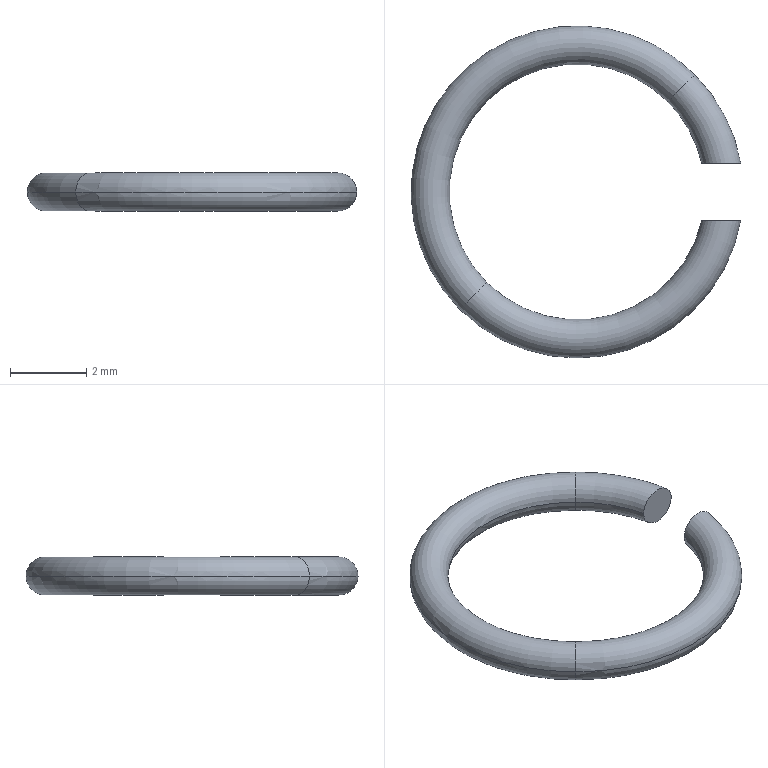Part | STEP file | ASND-0110-4216111400_AF0 | 1 solid | 8 faces | box 8.635 x 8.7 x 1 mm | volume 17.813 mm3 | torus 6 | plane 2
STEP:
#1=CARTESIAN_POINT('',(0.,0.,0.));
#2=DIRECTION('',(0.,0.,1.));
#3=DIRECTION('',(1.,0.,0.));
#4=AXIS2_PLACEMENT_3D('',#1,#2,#3);
#5=CARTESIAN_POINT('',(3.076,3.076,0.));
#6=VERTEX_POINT('',#5);
#7=CARTESIAN_POINT('',(2.369,2.369,0.));
#8=VERTEX_POINT('',#7);
#9=CARTESIAN_POINT('',(2.722,2.722,0.));
#10=DIRECTION('',(-0.7071,0.7071,0.));
#11=DIRECTION('',(-0.7071,-0.7071,0.));
#12=AXIS2_PLACEMENT_3D('',#9,#10,#11);
#13=CIRCLE('',#12,0.5);
#14=CARTESIAN_POINT('',(0.,0.,0.));
#15=DIRECTION('',(0.,0.,-1.));
#16=DIRECTION('',(0.7071,0.7071,0.));
#17=AXIS2_PLACEMENT_3D('',#14,#15,#16);
#18=TOROIDAL_SURFACE('',#17,3.85,0.5);
#19=CARTESIAN_POINT('',(0.,-3.142));
#20=DIRECTION('',(0.,1.));
#21=VECTOR('',#20,1.);
#22=LINE('',#19,#21);
#23=(GEOMETRIC_REPRESENTATION_CONTEXT(2)PARAMETRIC_REPRESENTATION_CONTEXT()REPRESENTATION_CONTEXT('',''));
#24=DEFINITIONAL_REPRESENTATION('',(#22),#23);
#25=PCURVE('',#18,#24);
#26=CARTESIAN_POINT('',(0.,0.,0.));
#27=DIRECTION('',(0.,0.,-1.));
#28=DIRECTION('',(0.7071,0.7071,0.));
#29=AXIS2_PLACEMENT_3D('',#26,#27,#28);
#30=TOROIDAL_SURFACE('',#29,3.85,0.5);
#31=CARTESIAN_POINT('',(6.283,-3.142));
#32=DIRECTION('',(0.,1.));
#33=VECTOR('',#32,1.);
#34=LINE('',#31,#33);
#35=(GEOMETRIC_REPRESENTATION_CONTEXT(2)PARAMETRIC_REPRESENTATION_CONTEXT()REPRESENTATION_CONTEXT('',''));
#36=DEFINITIONAL_REPRESENTATION('',(#34),#35);
#37=PCURVE('',#30,#36);
#38=SURFACE_CURVE('',#13,(#25,#37),.PCURVE_S1.);
#39=EDGE_CURVE('',#6,#8,#38,.T.);
#40=ORIENTED_EDGE('',*,*,#39,.F.);
#41=CARTESIAN_POINT('',(4.285,0.75,0.));
#42=VERTEX_POINT('',#41);
#43=CARTESIAN_POINT('',(0.,0.,0.));
#44=DIRECTION('',(0.,0.,-1.));
#45=DIRECTION('',(-1.,0.,0.));
#46=AXIS2_PLACEMENT_3D('',#43,#44,#45);
#47=CIRCLE('',#46,4.35);
#48=CARTESIAN_POINT('',(-2.356,0.));
#49=DIRECTION('',(1.,0.));
#50=VECTOR('',#49,1.);
#51=LINE('',#48,#50);
#52=(GEOMETRIC_REPRESENTATION_CONTEXT(2)PARAMETRIC_REPRESENTATION_CONTEXT()REPRESENTATION_CONTEXT('',''));
#53=DEFINITIONAL_REPRESENTATION('',(#51),#52);
#54=PCURVE('',#18,#53);
#55=CARTESIAN_POINT('',(0.,0.,0.));
#56=DIRECTION('',(0.,0.,-1.));
#57=DIRECTION('',(0.7071,0.7071,0.));
#58=AXIS2_PLACEMENT_3D('',#55,#56,#57);
#59=TOROIDAL_SURFACE('',#58,3.85,0.5);
#60=CARTESIAN_POINT('',(-2.356,6.283));
#61=DIRECTION('',(1.,0.));
#62=VECTOR('',#61,1.);
#63=LINE('',#60,#62);
#64=(GEOMETRIC_REPRESENTATION_CONTEXT(2)PARAMETRIC_REPRESENTATION_CONTEXT()REPRESENTATION_CONTEXT('',''));
#65=DEFINITIONAL_REPRESENTATION('',(#63),#64);
#66=PCURVE('',#59,#65);
#67=SURFACE_CURVE('',#47,(#54,#66),.PCURVE_S1.);
#68=EDGE_CURVE('',#6,#42,#67,.T.);
#69=ORIENTED_EDGE('',*,*,#68,.T.);
#70=CARTESIAN_POINT('',(3.776,0.75,-0.5));
#71=VERTEX_POINT('',#70);
#72=CARTESIAN_POINT('',(4.285,0.75,0.));
#73=CARTESIAN_POINT('',(4.285,0.75,-0.1146));
#74=CARTESIAN_POINT('',(4.242,0.7512,-0.2389));
#75=CARTESIAN_POINT('',(4.064,0.7514,-0.4328));
#76=CARTESIAN_POINT('',(3.926,0.75,-0.5));
#77=CARTESIAN_POINT('',(3.776,0.75,-0.5));
#78=B_SPLINE_CURVE_WITH_KNOTS('',3,(#72,#73,#74,#75,#76,#77),.UNSPECIFIED.,.F.,.F.,(4,2,4),(0.5,0.75,1.),.UNSPECIFIED.);
#79=CARTESIAN_POINT('',(0.6121,0.));
#80=CARTESIAN_POINT('',(0.6121,0.02083));
#81=CARTESIAN_POINT('',(0.6121,0.06282));
#82=CARTESIAN_POINT('',(0.6119,0.1267));
#83=CARTESIAN_POINT('',(0.6117,0.1915));
#84=CARTESIAN_POINT('',(0.6114,0.257));
#85=CARTESIAN_POINT('',(0.6109,0.3233));
#86=CARTESIAN_POINT('',(0.6104,0.3903));
#87=CARTESIAN_POINT('',(0.6098,0.4579));
#88=CARTESIAN_POINT('',(0.6091,0.5263));
#89=CARTESIAN_POINT('',(0.6083,0.5955));
#90=CARTESIAN_POINT('',(0.6074,0.6654));
#91=CARTESIAN_POINT('',(0.6064,0.7363));
#92=CARTESIAN_POINT('',(0.6054,0.8082));
#93=CARTESIAN_POINT('',(0.6042,0.881));
#94=CARTESIAN_POINT('',(0.6029,0.9547));
#95=CARTESIAN_POINT('',(0.6015,1.029));
#96=CARTESIAN_POINT('',(0.6001,1.104));
#97=CARTESIAN_POINT('',(0.5985,1.18));
#98=CARTESIAN_POINT('',(0.5969,1.257));
#99=CARTESIAN_POINT('',(0.5951,1.334));
#100=CARTESIAN_POINT('',(0.5933,1.412));
#101=CARTESIAN_POINT('',(0.5914,1.491));
#102=CARTESIAN_POINT('',(0.59,1.544));
#103=CARTESIAN_POINT('',(0.5893,1.571));
#104=B_SPLINE_CURVE_WITH_KNOTS('',3,(#79,#80,#81,#82,#83,#84,#85,#86,#87,#88,#89,#90,#91,#92,#93,#94,#95,#96,#97,#98,#99,#100,#101,#102,#103),.UNSPECIFIED.,.F.,.F.,(4,1,1,1,1,1,1,1,1,1,1,1,1,1,1,1,1,1,1,1,1,1,4),(0.5,0.5227,0.5455,0.5682,0.5909,0.6136,0.6364,0.6591,0.6818,0.7045,0.7273,0.75,0.7727,0.7955,0.8182,0.8409,0.8636,0.8864,0.9091,0.9318,0.9545,0.9773,1.),.QUASI_UNIFORM_KNOTS.);
#105=(GEOMETRIC_REPRESENTATION_CONTEXT(2)PARAMETRIC_REPRESENTATION_CONTEXT()REPRESENTATION_CONTEXT('',''));
#106=DEFINITIONAL_REPRESENTATION('',(#104),#105);
#107=PCURVE('',#18,#106);
#108=CARTESIAN_POINT('',(5.049,0.75,-1.526));
#109=DIRECTION('',(0.,1.,0.));
#110=DIRECTION('',(0.7071,0.,0.7071));
#111=AXIS2_PLACEMENT_3D('',#108,#109,#110);
#112=PLANE('',#111);
#113=CARTESIAN_POINT('',(0.5386,-1.619));
#114=CARTESIAN_POINT('',(0.4576,-1.538));
#115=CARTESIAN_POINT('',(0.3397,-1.48));
#116=CARTESIAN_POINT('',(0.07614,-1.469));
#117=CARTESIAN_POINT('',(-0.06847,-1.519));
#118=CARTESIAN_POINT('',(-0.1746,-1.625));
#119=B_SPLINE_CURVE_WITH_KNOTS('',3,(#113,#114,#115,#116,#117,#118),.UNSPECIFIED.,.F.,.F.,(4,2,4),(0.5,0.75,1.),.UNSPECIFIED.);
#120=(GEOMETRIC_REPRESENTATION_CONTEXT(2)PARAMETRIC_REPRESENTATION_CONTEXT()REPRESENTATION_CONTEXT('',''));
#121=DEFINITIONAL_REPRESENTATION('',(#119),#120);
#122=PCURVE('',#112,#121);
#123=SURFACE_CURVE('',#78,(#107,#122),.PCURVE_S1.);
#124=EDGE_CURVE('',#42,#71,#123,.T.);
#125=ORIENTED_EDGE('',*,*,#124,.T.);
#126=CARTESIAN_POINT('',(3.265,0.75,0.));
#127=VERTEX_POINT('',#126);
#128=CARTESIAN_POINT('',(3.776,0.75,-0.5));
#129=CARTESIAN_POINT('',(3.752,0.7499,-0.499));
#130=CARTESIAN_POINT('',(3.706,0.7499,-0.4972));
#131=CARTESIAN_POINT('',(3.642,0.7494,-0.4836));
#132=CARTESIAN_POINT('',(3.587,0.749,-0.4654));
#133=CARTESIAN_POINT('',(3.541,0.7488,-0.4445));
#134=CARTESIAN_POINT('',(3.503,0.7488,-0.4231));
#135=CARTESIAN_POINT('',(3.474,0.749,-0.4029));
#136=CARTESIAN_POINT('',(3.451,0.7493,-0.3853));
#137=CARTESIAN_POINT('',(3.434,0.7496,-0.3714));
#138=CARTESIAN_POINT('',(3.424,0.7499,-0.3617));
#139=CARTESIAN_POINT('',(3.384,0.7505,-0.3243));
#140=CARTESIAN_POINT('',(3.327,0.7495,-0.2494));
#141=CARTESIAN_POINT('',(3.274,0.7498,-0.1259));
#142=CARTESIAN_POINT('',(3.268,0.7499,-0.04095));
#143=CARTESIAN_POINT('',(3.265,0.75,0.));
#144=B_SPLINE_CURVE_WITH_KNOTS('',3,(#128,#129,#130,#131,#132,#133,#134,#135,#136,#137,#138,#139,#140,#141,#142,#143),.UNSPECIFIED.,.F.,.F.,(4,1,1,1,1,1,1,1,1,1,1,1,1,4),(0.,0.04566,0.08672,0.1232,0.1551,0.1824,0.2052,0.2234,0.237,0.246,0.2505,0.3396,0.4227,0.5),.UNSPECIFIED.);
#145=CARTESIAN_POINT('',(0.5893,1.571));
#146=CARTESIAN_POINT('',(0.5891,1.579));
#147=CARTESIAN_POINT('',(0.5887,1.594));
#148=CARTESIAN_POINT('',(0.5881,1.618));
#149=CARTESIAN_POINT('',(0.5875,1.642));
#150=CARTESIAN_POINT('',(0.5869,1.665));
#151=CARTESIAN_POINT('',(0.5863,1.689));
#152=CARTESIAN_POINT('',(0.5857,1.712));
#153=CARTESIAN_POINT('',(0.5851,1.736));
#154=CARTESIAN_POINT('',(0.5845,1.759));
#155=CARTESIAN_POINT('',(0.5839,1.783));
#156=CARTESIAN_POINT('',(0.5833,1.807));
#157=CARTESIAN_POINT('',(0.5826,1.83));
#158=CARTESIAN_POINT('',(0.582,1.854));
#159=CARTESIAN_POINT('',(0.5814,1.878));
#160=CARTESIAN_POINT('',(0.5808,1.901));
#161=CARTESIAN_POINT('',(0.5802,1.925));
#162=CARTESIAN_POINT('',(0.5796,1.948));
#163=CARTESIAN_POINT('',(0.579,1.972));
#164=CARTESIAN_POINT('',(0.5784,1.996));
#165=CARTESIAN_POINT('',(0.5778,2.019));
#166=CARTESIAN_POINT('',(0.5772,2.043));
#167=CARTESIAN_POINT('',(0.5766,2.066));
#168=CARTESIAN_POINT('',(0.576,2.09));
#169=CARTESIAN_POINT('',(0.5754,2.114));
#170=CARTESIAN_POINT('',(0.5748,2.137));
#171=CARTESIAN_POINT('',(0.5741,2.161));
#172=CARTESIAN_POINT('',(0.5735,2.185));
#173=CARTESIAN_POINT('',(0.5729,2.208));
#174=CARTESIAN_POINT('',(0.5723,2.232));
#175=CARTESIAN_POINT('',(0.5717,2.256));
#176=CARTESIAN_POINT('',(0.5711,2.279));
#177=CARTESIAN_POINT('',(0.5705,2.303));
#178=CARTESIAN_POINT('',(0.5699,2.326));
#179=CARTESIAN_POINT('',(0.5693,2.35));
#180=CARTESIAN_POINT('',(0.5688,2.374));
#181=CARTESIAN_POINT('',(0.5683,2.398));
#182=CARTESIAN_POINT('',(0.5677,2.421));
#183=CARTESIAN_POINT('',(0.5672,2.445));
#184=CARTESIAN_POINT('',(0.5668,2.469));
#185=CARTESIAN_POINT('',(0.5663,2.493));
#186=CARTESIAN_POINT('',(0.5659,2.517));
#187=CARTESIAN_POINT('',(0.5654,2.541));
#188=CARTESIAN_POINT('',(0.565,2.565));
#189=CARTESIAN_POINT('',(0.5646,2.589));
#190=CARTESIAN_POINT('',(0.5642,2.613));
#191=CARTESIAN_POINT('',(0.5639,2.637));
#192=CARTESIAN_POINT('',(0.5635,2.661));
#193=CARTESIAN_POINT('',(0.5631,2.685));
#194=CARTESIAN_POINT('',(0.5628,2.709));
#195=CARTESIAN_POINT('',(0.5625,2.733));
#196=CARTESIAN_POINT('',(0.5621,2.757));
#197=CARTESIAN_POINT('',(0.5618,2.781));
#198=CARTESIAN_POINT('',(0.5616,2.805));
#199=CARTESIAN_POINT('',(0.5613,2.829));
#200=CARTESIAN_POINT('',(0.5611,2.853));
#201=CARTESIAN_POINT('',(0.5608,2.877));
#202=CARTESIAN_POINT('',(0.5606,2.901));
#203=CARTESIAN_POINT('',(0.5605,2.925));
#204=CARTESIAN_POINT('',(0.5603,2.949));
#205=CARTESIAN_POINT('',(0.5602,2.973));
#206=CARTESIAN_POINT('',(0.5601,2.997));
#207=CARTESIAN_POINT('',(0.56,3.021));
#208=CARTESIAN_POINT('',(0.5599,3.045));
#209=CARTESIAN_POINT('',(0.5598,3.069));
#210=CARTESIAN_POINT('',(0.5597,3.093));
#211=CARTESIAN_POINT('',(0.5597,3.117));
#212=CARTESIAN_POINT('',(0.5596,3.134));
#213=CARTESIAN_POINT('',(0.5596,3.142));
#214=B_SPLINE_CURVE_WITH_KNOTS('',3,(#145,#146,#147,#148,#149,#150,#151,#152,#153,#154,#155,#156,#157,#158,#159,#160,#161,#162,#163,#164,#165,#166,#167,#168,#169,#170,#171,#172,#173,#174,#175,#176,#177,#178,#179,#180,#181,#182,#183,#184,#185,#186,#187,#188,#189,#190,#191,#192,#193,#194,#195,#196,#197,#198,#199,#200,#201,#202,#203,#204,#205,#206,#207,#208,#209,#210,#211,#212,#213),.UNSPECIFIED.,.F.,.F.,(4,1,1,1,1,1,1,1,1,1,1,1,1,1,1,1,1,1,1,1,1,1,1,1,1,1,1,1,1,1,1,1,1,1,1,1,1,1,1,1,1,1,1,1,1,1,1,1,1,1,1,1,1,1,1,1,1,1,1,1,1,1,1,1,1,1,4),(0.,0.007576,0.01515,0.02273,0.0303,0.03788,0.04545,0.05303,0.06061,0.06818,0.07576,0.08333,0.09091,0.09848,0.1061,0.1136,0.1212,0.1288,0.1364,0.1439,0.1515,0.1591,0.1667,0.1742,0.1818,0.1894,0.197,0.2045,0.2121,0.2197,0.2273,0.2348,0.2424,0.25,0.2576,0.2652,0.2727,0.2803,0.2879,0.2955,0.303,0.3106,0.3182,0.3258,0.3333,0.3409,0.3485,0.3561,0.3636,0.3712,0.3788,0.3864,0.3939,0.4015,0.4091,0.4167,0.4242,0.4318,0.4394,0.447,0.4545,0.4621,0.4697,0.4773,0.4848,0.4924,0.5),.QUASI_UNIFORM_KNOTS.);
#215=(GEOMETRIC_REPRESENTATION_CONTEXT(2)PARAMETRIC_REPRESENTATION_CONTEXT()REPRESENTATION_CONTEXT('',''));
#216=DEFINITIONAL_REPRESENTATION('',(#214),#215);
#217=PCURVE('',#18,#216);
#218=CARTESIAN_POINT('',(-0.1746,-1.625));
#219=CARTESIAN_POINT('',(-0.191,-1.643));
#220=CARTESIAN_POINT('',(-0.2221,-1.676));
#221=CARTESIAN_POINT('',(-0.2577,-1.731));
#222=CARTESIAN_POINT('',(-0.2838,-1.783));
#223=CARTESIAN_POINT('',(-0.3016,-1.83));
#224=CARTESIAN_POINT('',(-0.3131,-1.872));
#225=CARTESIAN_POINT('',(-0.32,-1.908));
#226=CARTESIAN_POINT('',(-0.3238,-1.936));
#227=CARTESIAN_POINT('',(-0.3255,-1.958));
#228=CARTESIAN_POINT('',(-0.3262,-1.972));
#229=CARTESIAN_POINT('',(-0.3275,-2.026));
#230=CARTESIAN_POINT('',(-0.3154,-2.12));
#231=CARTESIAN_POINT('',(-0.265,-2.244));
#232=CARTESIAN_POINT('',(-0.2094,-2.309));
#233=CARTESIAN_POINT('',(-0.1826,-2.34));
#234=B_SPLINE_CURVE_WITH_KNOTS('',3,(#218,#219,#220,#221,#222,#223,#224,#225,#226,#227,#228,#229,#230,#231,#232,#233),.UNSPECIFIED.,.F.,.F.,(4,1,1,1,1,1,1,1,1,1,1,1,1,4),(0.,0.04566,0.08672,0.1232,0.1551,0.1824,0.2052,0.2234,0.237,0.246,0.2505,0.3396,0.4227,0.5),.UNSPECIFIED.);
#235=(GEOMETRIC_REPRESENTATION_CONTEXT(2)PARAMETRIC_REPRESENTATION_CONTEXT()REPRESENTATION_CONTEXT('',''));
#236=DEFINITIONAL_REPRESENTATION('',(#234),#235);
#237=PCURVE('',#112,#236);
#238=SURFACE_CURVE('',#144,(#217,#237),.PCURVE_S1.);
#239=EDGE_CURVE('',#71,#127,#238,.T.);
#240=ORIENTED_EDGE('',*,*,#239,.T.);
#241=CARTESIAN_POINT('',(0.,0.,0.));
#242=DIRECTION('',(0.,0.,-1.));
#243=DIRECTION('',(-1.,0.,0.));
#244=AXIS2_PLACEMENT_3D('',#241,#242,#243);
#245=CIRCLE('',#244,3.35);
#246=CARTESIAN_POINT('',(-2.356,3.142));
#247=DIRECTION('',(1.,0.));
#248=VECTOR('',#247,1.);
#249=LINE('',#246,#248);
#250=(GEOMETRIC_REPRESENTATION_CONTEXT(2)PARAMETRIC_REPRESENTATION_CONTEXT()REPRESENTATION_CONTEXT('',''));
#251=DEFINITIONAL_REPRESENTATION('',(#249),#250);
#252=PCURVE('',#18,#251);
#253=CARTESIAN_POINT('',(-2.356,3.142));
#254=DIRECTION('',(1.,0.));
#255=VECTOR('',#254,1.);
#256=LINE('',#253,#255);
#257=(GEOMETRIC_REPRESENTATION_CONTEXT(2)PARAMETRIC_REPRESENTATION_CONTEXT()REPRESENTATION_CONTEXT('',''));
#258=DEFINITIONAL_REPRESENTATION('',(#256),#257);
#259=PCURVE('',#59,#258);
#260=SURFACE_CURVE('',#245,(#252,#259),.PCURVE_S1.);
#261=EDGE_CURVE('',#8,#127,#260,.T.);
#262=ORIENTED_EDGE('',*,*,#261,.F.);
#263=EDGE_LOOP('',(#40,#69,#125,#240,#262));
#264=FACE_BOUND('',#263,.T.);
#265=ADVANCED_FACE('',(#264),#18,.T.);
#266=CARTESIAN_POINT('',(-3.076,-3.076,0.));
#267=VERTEX_POINT('',#266);
#268=CARTESIAN_POINT('',(-2.369,-2.369,0.));
#269=VERTEX_POINT('',#268);
#270=CARTESIAN_POINT('',(-2.722,-2.722,0.));
#271=DIRECTION('',(0.7071,-0.7071,0.));
#272=DIRECTION('',(0.7071,0.7071,0.));
#273=AXIS2_PLACEMENT_3D('',#270,#271,#272);
#274=CIRCLE('',#273,0.5);
#275=CARTESIAN_POINT('',(3.142,-3.142));
#276=DIRECTION('',(0.,1.));
#277=VECTOR('',#276,1.);
#278=LINE('',#275,#277);
#279=(GEOMETRIC_REPRESENTATION_CONTEXT(2)PARAMETRIC_REPRESENTATION_CONTEXT()REPRESENTATION_CONTEXT('',''));
#280=DEFINITIONAL_REPRESENTATION('',(#278),#279);
#281=PCURVE('',#30,#280);
#282=CARTESIAN_POINT('',(0.,0.,0.));
#283=DIRECTION('',(0.,0.,-1.));
#284=DIRECTION('',(0.7071,0.7071,0.));
#285=AXIS2_PLACEMENT_3D('',#282,#283,#284);
#286=TOROIDAL_SURFACE('',#285,3.85,0.5);
#287=CARTESIAN_POINT('',(3.142,-3.142));
#288=DIRECTION('',(0.,1.));
#289=VECTOR('',#288,1.);
#290=LINE('',#287,#289);
#291=(GEOMETRIC_REPRESENTATION_CONTEXT(2)PARAMETRIC_REPRESENTATION_CONTEXT()REPRESENTATION_CONTEXT('',''));
#292=DEFINITIONAL_REPRESENTATION('',(#290),#291);
#293=PCURVE('',#286,#292);
#294=SURFACE_CURVE('',#274,(#281,#293),.PCURVE_S1.);
#295=EDGE_CURVE('',#267,#269,#294,.T.);
#296=ORIENTED_EDGE('',*,*,#295,.F.);
#297=CARTESIAN_POINT('',(0.,0.,0.));
#298=DIRECTION('',(0.,0.,-1.));
#299=DIRECTION('',(-1.,0.,0.));
#300=AXIS2_PLACEMENT_3D('',#297,#298,#299);
#301=CIRCLE('',#300,4.35);
#302=CARTESIAN_POINT('',(-2.356,0.));
#303=DIRECTION('',(1.,0.));
#304=VECTOR('',#303,1.);
#305=LINE('',#302,#304);
#306=(GEOMETRIC_REPRESENTATION_CONTEXT(2)PARAMETRIC_REPRESENTATION_CONTEXT()REPRESENTATION_CONTEXT('',''));
#307=DEFINITIONAL_REPRESENTATION('',(#305),#306);
#308=PCURVE('',#30,#307);
#309=CARTESIAN_POINT('',(0.,0.,0.));
#310=DIRECTION('',(0.,0.,-1.));
#311=DIRECTION('',(0.7071,0.7071,0.));
#312=AXIS2_PLACEMENT_3D('',#309,#310,#311);
#313=TOROIDAL_SURFACE('',#312,3.85,0.5);
#314=CARTESIAN_POINT('',(-2.356,6.283));
#315=DIRECTION('',(1.,0.));
#316=VECTOR('',#315,1.);
#317=LINE('',#314,#316);
#318=(GEOMETRIC_REPRESENTATION_CONTEXT(2)PARAMETRIC_REPRESENTATION_CONTEXT()REPRESENTATION_CONTEXT('',''));
#319=DEFINITIONAL_REPRESENTATION('',(#317),#318);
#320=PCURVE('',#313,#319);
#321=SURFACE_CURVE('',#301,(#308,#320),.PCURVE_S1.);
#322=EDGE_CURVE('',#267,#6,#321,.T.);
#323=ORIENTED_EDGE('',*,*,#322,.T.);
#324=ORIENTED_EDGE('',*,*,#39,.T.);
#325=CARTESIAN_POINT('',(0.,0.,0.));
#326=DIRECTION('',(0.,0.,-1.));
#327=DIRECTION('',(-1.,0.,0.));
#328=AXIS2_PLACEMENT_3D('',#325,#326,#327);
#329=CIRCLE('',#328,3.35);
#330=CARTESIAN_POINT('',(-2.356,3.142));
#331=DIRECTION('',(1.,0.));
#332=VECTOR('',#331,1.);
#333=LINE('',#330,#332);
#334=(GEOMETRIC_REPRESENTATION_CONTEXT(2)PARAMETRIC_REPRESENTATION_CONTEXT()REPRESENTATION_CONTEXT('',''));
#335=DEFINITIONAL_REPRESENTATION('',(#333),#334);
#336=PCURVE('',#30,#335);
#337=CARTESIAN_POINT('',(-2.356,3.142));
#338=DIRECTION('',(1.,0.));
#339=VECTOR('',#338,1.);
#340=LINE('',#337,#339);
#341=(GEOMETRIC_REPRESENTATION_CONTEXT(2)PARAMETRIC_REPRESENTATION_CONTEXT()REPRESENTATION_CONTEXT('',''));
#342=DEFINITIONAL_REPRESENTATION('',(#340),#341);
#343=PCURVE('',#313,#342);
#344=SURFACE_CURVE('',#329,(#336,#343),.PCURVE_S1.);
#345=EDGE_CURVE('',#269,#8,#344,.T.);
#346=ORIENTED_EDGE('',*,*,#345,.F.);
#347=EDGE_LOOP('',(#296,#323,#324,#346));
#348=FACE_BOUND('',#347,.T.);
#349=ADVANCED_FACE('',(#348),#30,.T.);
#350=CARTESIAN_POINT('',(3.776,-0.75,-0.5));
#351=VERTEX_POINT('',#350);
#352=CARTESIAN_POINT('',(4.285,-0.75,0.));
#353=VERTEX_POINT('',#352);
#354=CARTESIAN_POINT('',(3.776,-0.75,-0.5));
#355=CARTESIAN_POINT('',(3.926,-0.75,-0.5));
#356=CARTESIAN_POINT('',(4.064,-0.7514,-0.4328));
#357=CARTESIAN_POINT('',(4.242,-0.7512,-0.2389));
#358=CARTESIAN_POINT('',(4.285,-0.75,-0.1146));
#359=CARTESIAN_POINT('',(4.285,-0.75,0.));
#360=B_SPLINE_CURVE_WITH_KNOTS('',3,(#354,#355,#356,#357,#358,#359),.UNSPECIFIED.,.F.,.F.,(4,2,4),(0.,0.25,0.5),.UNSPECIFIED.);
#361=CARTESIAN_POINT('',(0.9815,1.571));
#362=CARTESIAN_POINT('',(0.9808,1.544));
#363=CARTESIAN_POINT('',(0.9794,1.491));
#364=CARTESIAN_POINT('',(0.9775,1.412));
#365=CARTESIAN_POINT('',(0.9757,1.334));
#366=CARTESIAN_POINT('',(0.9739,1.257));
#367=CARTESIAN_POINT('',(0.9723,1.18));
#368=CARTESIAN_POINT('',(0.9707,1.105));
#369=CARTESIAN_POINT('',(0.9693,1.029));
#370=CARTESIAN_POINT('',(0.9679,0.9548));
#371=CARTESIAN_POINT('',(0.9666,0.8811));
#372=CARTESIAN_POINT('',(0.9654,0.8083));
#373=CARTESIAN_POINT('',(0.9644,0.7364));
#374=CARTESIAN_POINT('',(0.9634,0.6655));
#375=CARTESIAN_POINT('',(0.9625,0.5956));
#376=CARTESIAN_POINT('',(0.9617,0.5264));
#377=CARTESIAN_POINT('',(0.961,0.458));
#378=CARTESIAN_POINT('',(0.9604,0.3903));
#379=CARTESIAN_POINT('',(0.9599,0.3233));
#380=CARTESIAN_POINT('',(0.9594,0.257));
#381=CARTESIAN_POINT('',(0.9591,0.1915));
#382=CARTESIAN_POINT('',(0.9589,0.1267));
#383=CARTESIAN_POINT('',(0.9587,0.06282));
#384=CARTESIAN_POINT('',(0.9587,0.02083));
#385=CARTESIAN_POINT('',(0.9587,0.));
#386=B_SPLINE_CURVE_WITH_KNOTS('',3,(#361,#362,#363,#364,#365,#366,#367,#368,#369,#370,#371,#372,#373,#374,#375,#376,#377,#378,#379,#380,#381,#382,#383,#384,#385),.UNSPECIFIED.,.F.,.F.,(4,1,1,1,1,1,1,1,1,1,1,1,1,1,1,1,1,1,1,1,1,1,4),(0.,0.02273,0.04545,0.06818,0.09091,0.1136,0.1364,0.1591,0.1818,0.2045,0.2273,0.25,0.2727,0.2955,0.3182,0.3409,0.3636,0.3864,0.4091,0.4318,0.4545,0.4773,0.5),.QUASI_UNIFORM_KNOTS.);
#387=(GEOMETRIC_REPRESENTATION_CONTEXT(2)PARAMETRIC_REPRESENTATION_CONTEXT()REPRESENTATION_CONTEXT('',''));
#388=DEFINITIONAL_REPRESENTATION('',(#386),#387);
#389=PCURVE('',#286,#388);
#390=CARTESIAN_POINT('',(2.042,-0.75,-1.526));
#391=DIRECTION('',(0.,-1.,0.));
#392=DIRECTION('',(0.7071,0.,0.7071));
#393=AXIS2_PLACEMENT_3D('',#390,#391,#392);
#394=PLANE('',#393);
#395=CARTESIAN_POINT('',(1.951,-0.501));
#396=CARTESIAN_POINT('',(2.057,-0.6071));
#397=CARTESIAN_POINT('',(2.202,-0.6567));
#398=CARTESIAN_POINT('',(2.465,-0.646));
#399=CARTESIAN_POINT('',(2.583,-0.5881));
#400=CARTESIAN_POINT('',(2.664,-0.5071));
#401=B_SPLINE_CURVE_WITH_KNOTS('',3,(#395,#396,#397,#398,#399,#400),.UNSPECIFIED.,.F.,.F.,(4,2,4),(0.,0.25,0.5),.UNSPECIFIED.);
#402=(GEOMETRIC_REPRESENTATION_CONTEXT(2)PARAMETRIC_REPRESENTATION_CONTEXT()REPRESENTATION_CONTEXT('',''));
#403=DEFINITIONAL_REPRESENTATION('',(#401),#402);
#404=PCURVE('',#394,#403);
#405=SURFACE_CURVE('',#360,(#389,#404),.PCURVE_S1.);
#406=EDGE_CURVE('',#351,#353,#405,.T.);
#407=ORIENTED_EDGE('',*,*,#406,.T.);
#408=CARTESIAN_POINT('',(0.,0.,0.));
#409=DIRECTION('',(0.,0.,-1.));
#410=DIRECTION('',(-1.,0.,0.));
#411=AXIS2_PLACEMENT_3D('',#408,#409,#410);
#412=CIRCLE('',#411,4.35);
#413=CARTESIAN_POINT('',(-2.356,0.));
#414=DIRECTION('',(1.,0.));
#415=VECTOR('',#414,1.);
#416=LINE('',#413,#415);
#417=(GEOMETRIC_REPRESENTATION_CONTEXT(2)PARAMETRIC_REPRESENTATION_CONTEXT()REPRESENTATION_CONTEXT('',''));
#418=DEFINITIONAL_REPRESENTATION('',(#416),#417);
#419=PCURVE('',#286,#418);
#420=CARTESIAN_POINT('',(0.,0.,0.));
#421=DIRECTION('',(0.,0.,-1.));
#422=DIRECTION('',(0.7071,0.7071,0.));
#423=AXIS2_PLACEMENT_3D('',#420,#421,#422);
#424=TOROIDAL_SURFACE('',#423,3.85,0.5);
#425=CARTESIAN_POINT('',(-2.356,6.283));
#426=DIRECTION('',(1.,0.));
#427=VECTOR('',#426,1.);
#428=LINE('',#425,#427);
#429=(GEOMETRIC_REPRESENTATION_CONTEXT(2)PARAMETRIC_REPRESENTATION_CONTEXT()REPRESENTATION_CONTEXT('',''));
#430=DEFINITIONAL_REPRESENTATION('',(#428),#429);
#431=PCURVE('',#424,#430);
#432=SURFACE_CURVE('',#412,(#419,#431),.PCURVE_S1.);
#433=EDGE_CURVE('',#353,#267,#432,.T.);
#434=ORIENTED_EDGE('',*,*,#433,.T.);
#435=ORIENTED_EDGE('',*,*,#295,.T.);
#436=CARTESIAN_POINT('',(3.265,-0.75,0.));
#437=VERTEX_POINT('',#436);
#438=CARTESIAN_POINT('',(0.,0.,0.));
#439=DIRECTION('',(0.,0.,-1.));
#440=DIRECTION('',(-1.,0.,0.));
#441=AXIS2_PLACEMENT_3D('',#438,#439,#440);
#442=CIRCLE('',#441,3.35);
#443=CARTESIAN_POINT('',(-2.356,3.142));
#444=DIRECTION('',(1.,0.));
#445=VECTOR('',#444,1.);
#446=LINE('',#443,#445);
#447=(GEOMETRIC_REPRESENTATION_CONTEXT(2)PARAMETRIC_REPRESENTATION_CONTEXT()REPRESENTATION_CONTEXT('',''));
#448=DEFINITIONAL_REPRESENTATION('',(#446),#447);
#449=PCURVE('',#286,#448);
#450=CARTESIAN_POINT('',(-2.356,3.142));
#451=DIRECTION('',(1.,0.));
#452=VECTOR('',#451,1.);
#453=LINE('',#450,#452);
#454=(GEOMETRIC_REPRESENTATION_CONTEXT(2)PARAMETRIC_REPRESENTATION_CONTEXT()REPRESENTATION_CONTEXT('',''));
#455=DEFINITIONAL_REPRESENTATION('',(#453),#454);
#456=PCURVE('',#424,#455);
#457=SURFACE_CURVE('',#442,(#449,#456),.PCURVE_S1.);
#458=EDGE_CURVE('',#437,#269,#457,.T.);
#459=ORIENTED_EDGE('',*,*,#458,.F.);
#460=CARTESIAN_POINT('',(3.265,-0.75,0.));
#461=CARTESIAN_POINT('',(3.266,-0.75,-0.02009));
#462=CARTESIAN_POINT('',(3.267,-0.7499,-0.06104));
#463=CARTESIAN_POINT('',(3.279,-0.7498,-0.1226));
#464=CARTESIAN_POINT('',(3.3,-0.7497,-0.1844));
#465=CARTESIAN_POINT('',(3.329,-0.7498,-0.245));
#466=CARTESIAN_POINT('',(3.368,-0.7499,-0.3032));
#467=CARTESIAN_POINT('',(3.423,-0.7503,-0.365));
#468=CARTESIAN_POINT('',(3.546,-0.7476,-0.4638));
#469=CARTESIAN_POINT('',(3.68,-0.749,-0.4848));
#470=CARTESIAN_POINT('',(3.776,-0.75,-0.5));
#471=B_SPLINE_CURVE_WITH_KNOTS('',3,(#460,#461,#462,#463,#464,#465,#466,#467,#468,#469,#470),.UNSPECIFIED.,.F.,.F.,(4,1,1,1,1,1,1,1,4),(0.5,0.5381,0.5777,0.6188,0.6613,0.7054,0.751,0.8192,1.),.UNSPECIFIED.);
#472=CARTESIAN_POINT('',(1.011,3.142));
#473=CARTESIAN_POINT('',(1.011,3.13));
#474=CARTESIAN_POINT('',(1.011,3.106));
#475=CARTESIAN_POINT('',(1.011,3.07));
#476=CARTESIAN_POINT('',(1.011,3.034));
#477=CARTESIAN_POINT('',(1.011,2.998));
#478=CARTESIAN_POINT('',(1.011,2.962));
#479=CARTESIAN_POINT('',(1.01,2.926));
#480=CARTESIAN_POINT('',(1.01,2.89));
#481=CARTESIAN_POINT('',(1.01,2.854));
#482=CARTESIAN_POINT('',(1.009,2.819));
#483=CARTESIAN_POINT('',(1.009,2.783));
#484=CARTESIAN_POINT('',(1.009,2.747));
#485=CARTESIAN_POINT('',(1.008,2.711));
#486=CARTESIAN_POINT('',(1.008,2.675));
#487=CARTESIAN_POINT('',(1.007,2.64));
#488=CARTESIAN_POINT('',(1.006,2.604));
#489=CARTESIAN_POINT('',(1.006,2.568));
#490=CARTESIAN_POINT('',(1.005,2.533));
#491=CARTESIAN_POINT('',(1.005,2.497));
#492=CARTESIAN_POINT('',(1.004,2.461));
#493=CARTESIAN_POINT('',(1.003,2.426));
#494=CARTESIAN_POINT('',(1.002,2.39));
#495=CARTESIAN_POINT('',(1.002,2.355));
#496=CARTESIAN_POINT('',(1.001,2.319));
#497=CARTESIAN_POINT('',(0.9999,2.284));
#498=CARTESIAN_POINT('',(0.999,2.248));
#499=CARTESIAN_POINT('',(0.998,2.213));
#500=CARTESIAN_POINT('',(0.9971,2.177));
#501=CARTESIAN_POINT('',(0.9962,2.142));
#502=CARTESIAN_POINT('',(0.9952,2.107));
#503=CARTESIAN_POINT('',(0.9943,2.073));
#504=CARTESIAN_POINT('',(0.9933,2.038));
#505=CARTESIAN_POINT('',(0.9924,2.003));
#506=CARTESIAN_POINT('',(0.9915,1.968));
#507=CARTESIAN_POINT('',(0.9905,1.932));
#508=CARTESIAN_POINT('',(0.9896,1.897));
#509=CARTESIAN_POINT('',(0.9887,1.861));
#510=CARTESIAN_POINT('',(0.9877,1.825));
#511=CARTESIAN_POINT('',(0.9868,1.789));
#512=CARTESIAN_POINT('',(0.9859,1.752));
#513=CARTESIAN_POINT('',(0.985,1.716));
#514=CARTESIAN_POINT('',(0.9841,1.68));
#515=CARTESIAN_POINT('',(0.9832,1.643));
#516=CARTESIAN_POINT('',(0.9823,1.607));
#517=CARTESIAN_POINT('',(0.9817,1.583));
#518=CARTESIAN_POINT('',(0.9815,1.571));
#519=B_SPLINE_CURVE_WITH_KNOTS('',3,(#472,#473,#474,#475,#476,#477,#478,#479,#480,#481,#482,#483,#484,#485,#486,#487,#488,#489,#490,#491,#492,#493,#494,#495,#496,#497,#498,#499,#500,#501,#502,#503,#504,#505,#506,#507,#508,#509,#510,#511,#512,#513,#514,#515,#516,#517,#518),.UNSPECIFIED.,.F.,.F.,(4,1,1,1,1,1,1,1,1,1,1,1,1,1,1,1,1,1,1,1,1,1,1,1,1,1,1,1,1,1,1,1,1,1,1,1,1,1,1,1,1,1,1,1,4),(0.5,0.5114,0.5227,0.5341,0.5455,0.5568,0.5682,0.5795,0.5909,0.6023,0.6136,0.625,0.6364,0.6477,0.6591,0.6705,0.6818,0.6932,0.7045,0.7159,0.7273,0.7386,0.75,0.7614,0.7727,0.7841,0.7955,0.8068,0.8182,0.8295,0.8409,0.8523,0.8636,0.875,0.8864,0.8977,0.9091,0.9205,0.9318,0.9432,0.9545,0.9659,0.9773,0.9886,1.),.QUASI_UNIFORM_KNOTS.);
#520=(GEOMETRIC_REPRESENTATION_CONTEXT(2)PARAMETRIC_REPRESENTATION_CONTEXT()REPRESENTATION_CONTEXT('',''));
#521=DEFINITIONAL_REPRESENTATION('',(#519),#520);
#522=PCURVE('',#286,#521);
#523=CARTESIAN_POINT('',(1.943,0.2141));
#524=CARTESIAN_POINT('',(1.93,0.1994));
#525=CARTESIAN_POINT('',(1.902,0.1694));
#526=CARTESIAN_POINT('',(1.867,0.1172));
#527=CARTESIAN_POINT('',(1.837,0.05924));
#528=CARTESIAN_POINT('',(1.815,-0.004466));
#529=CARTESIAN_POINT('',(1.802,-0.073));
#530=CARTESIAN_POINT('',(1.797,-0.1561));
#531=CARTESIAN_POINT('',(1.814,-0.313));
#532=CARTESIAN_POINT('',(1.894,-0.4219));
#533=CARTESIAN_POINT('',(1.951,-0.501));
#534=B_SPLINE_CURVE_WITH_KNOTS('',3,(#523,#524,#525,#526,#527,#528,#529,#530,#531,#532,#533),.UNSPECIFIED.,.F.,.F.,(4,1,1,1,1,1,1,1,4),(0.5,0.5381,0.5777,0.6188,0.6613,0.7054,0.751,0.8192,1.),.UNSPECIFIED.);
#535=(GEOMETRIC_REPRESENTATION_CONTEXT(2)PARAMETRIC_REPRESENTATION_CONTEXT()REPRESENTATION_CONTEXT('',''));
#536=DEFINITIONAL_REPRESENTATION('',(#534),#535);
#537=PCURVE('',#394,#536);
#538=SURFACE_CURVE('',#471,(#522,#537),.PCURVE_S1.);
#539=EDGE_CURVE('',#437,#351,#538,.T.);
#540=ORIENTED_EDGE('',*,*,#539,.T.);
#541=EDGE_LOOP('',(#407,#434,#435,#459,#540));
#542=FACE_BOUND('',#541,.T.);
#543=ADVANCED_FACE('',(#542),#286,.T.);
#544=ORIENTED_EDGE('',*,*,#433,.F.);
#545=CARTESIAN_POINT('',(3.776,-0.75,0.5));
#546=VERTEX_POINT('',#545);
#547=CARTESIAN_POINT('',(4.285,-0.75,0.));
#548=CARTESIAN_POINT('',(4.285,-0.75,0.1146));
#549=CARTESIAN_POINT('',(4.242,-0.7512,0.2389));
#550=CARTESIAN_POINT('',(4.064,-0.7514,0.4328));
#551=CARTESIAN_POINT('',(3.926,-0.75,0.5));
#552=CARTESIAN_POINT('',(3.776,-0.75,0.5));
#553=B_SPLINE_CURVE_WITH_KNOTS('',3,(#547,#548,#549,#550,#551,#552),.UNSPECIFIED.,.F.,.F.,(4,2,4),(0.5,0.75,1.),.UNSPECIFIED.);
#554=CARTESIAN_POINT('',(0.9587,6.283));
#555=CARTESIAN_POINT('',(0.9587,6.262));
#556=CARTESIAN_POINT('',(0.9587,6.22));
#557=CARTESIAN_POINT('',(0.9589,6.156));
#558=CARTESIAN_POINT('',(0.9591,6.092));
#559=CARTESIAN_POINT('',(0.9594,6.026));
#560=CARTESIAN_POINT('',(0.9598,5.96));
#561=CARTESIAN_POINT('',(0.9604,5.893));
#562=CARTESIAN_POINT('',(0.961,5.825));
#563=CARTESIAN_POINT('',(0.9617,5.757));
#564=CARTESIAN_POINT('',(0.9625,5.688));
#565=CARTESIAN_POINT('',(0.9634,5.618));
#566=CARTESIAN_POINT('',(0.9644,5.547));
#567=CARTESIAN_POINT('',(0.9654,5.475));
#568=CARTESIAN_POINT('',(0.9666,5.402));
#569=CARTESIAN_POINT('',(0.9679,5.329));
#570=CARTESIAN_POINT('',(0.9692,5.254));
#571=CARTESIAN_POINT('',(0.9707,5.179));
#572=CARTESIAN_POINT('',(0.9723,5.103));
#573=CARTESIAN_POINT('',(0.9739,5.026));
#574=CARTESIAN_POINT('',(0.9757,4.949));
#575=CARTESIAN_POINT('',(0.9775,4.871));
#576=CARTESIAN_POINT('',(0.9794,4.792));
#577=CARTESIAN_POINT('',(0.9808,4.739));
#578=CARTESIAN_POINT('',(0.9815,4.712));
#579=B_SPLINE_CURVE_WITH_KNOTS('',3,(#554,#555,#556,#557,#558,#559,#560,#561,#562,#563,#564,#565,#566,#567,#568,#569,#570,#571,#572,#573,#574,#575,#576,#577,#578),.UNSPECIFIED.,.F.,.F.,(4,1,1,1,1,1,1,1,1,1,1,1,1,1,1,1,1,1,1,1,1,1,4),(0.5,0.5227,0.5455,0.5682,0.5909,0.6136,0.6364,0.6591,0.6818,0.7045,0.7273,0.75,0.7727,0.7955,0.8182,0.8409,0.8636,0.8864,0.9091,0.9318,0.9545,0.9773,1.),.QUASI_UNIFORM_KNOTS.);
#580=(GEOMETRIC_REPRESENTATION_CONTEXT(2)PARAMETRIC_REPRESENTATION_CONTEXT()REPRESENTATION_CONTEXT('',''));
#581=DEFINITIONAL_REPRESENTATION('',(#579),#580);
#582=PCURVE('',#424,#581);
#583=CARTESIAN_POINT('',(2.664,-0.5071));
#584=CARTESIAN_POINT('',(2.745,-0.4261));
#585=CARTESIAN_POINT('',(2.803,-0.3082));
#586=CARTESIAN_POINT('',(2.814,-0.04462));
#587=CARTESIAN_POINT('',(2.765,0.09999));
#588=CARTESIAN_POINT('',(2.658,0.2061));
#589=B_SPLINE_CURVE_WITH_KNOTS('',3,(#583,#584,#585,#586,#587,#588),.UNSPECIFIED.,.F.,.F.,(4,2,4),(0.5,0.75,1.),.UNSPECIFIED.);
#590=(GEOMETRIC_REPRESENTATION_CONTEXT(2)PARAMETRIC_REPRESENTATION_CONTEXT()REPRESENTATION_CONTEXT('',''));
#591=DEFINITIONAL_REPRESENTATION('',(#589),#590);
#592=PCURVE('',#394,#591);
#593=SURFACE_CURVE('',#553,(#582,#592),.PCURVE_S1.);
#594=EDGE_CURVE('',#353,#546,#593,.T.);
#595=ORIENTED_EDGE('',*,*,#594,.T.);
#596=CARTESIAN_POINT('',(3.776,-0.75,0.5));
#597=CARTESIAN_POINT('',(3.752,-0.7499,0.499));
#598=CARTESIAN_POINT('',(3.706,-0.7499,0.4972));
#599=CARTESIAN_POINT('',(3.642,-0.7494,0.4836));
#600=CARTESIAN_POINT('',(3.587,-0.749,0.4654));
#601=CARTESIAN_POINT('',(3.541,-0.7488,0.4445));
#602=CARTESIAN_POINT('',(3.503,-0.7488,0.4231));
#603=CARTESIAN_POINT('',(3.474,-0.749,0.4029));
#604=CARTESIAN_POINT('',(3.451,-0.7493,0.3853));
#605=CARTESIAN_POINT('',(3.434,-0.7496,0.3714));
#606=CARTESIAN_POINT('',(3.424,-0.7499,0.3617));
#607=CARTESIAN_POINT('',(3.384,-0.7505,0.3243));
#608=CARTESIAN_POINT('',(3.327,-0.7495,0.2494));
#609=CARTESIAN_POINT('',(3.274,-0.7498,0.1259));
#610=CARTESIAN_POINT('',(3.268,-0.7499,0.04095));
#611=CARTESIAN_POINT('',(3.265,-0.75,0.));
#612=B_SPLINE_CURVE_WITH_KNOTS('',3,(#596,#597,#598,#599,#600,#601,#602,#603,#604,#605,#606,#607,#608,#609,#610,#611),.UNSPECIFIED.,.F.,.F.,(4,1,1,1,1,1,1,1,1,1,1,1,1,4),(0.,0.04566,0.08672,0.1232,0.1551,0.1824,0.2052,0.2234,0.237,0.246,0.2505,0.3396,0.4227,0.5),.UNSPECIFIED.);
#613=CARTESIAN_POINT('',(0.9815,4.712));
#614=CARTESIAN_POINT('',(0.9817,4.705));
#615=CARTESIAN_POINT('',(0.9821,4.689));
#616=CARTESIAN_POINT('',(0.9827,4.665));
#617=CARTESIAN_POINT('',(0.9833,4.642));
#618=CARTESIAN_POINT('',(0.9839,4.618));
#619=CARTESIAN_POINT('',(0.9845,4.594));
#620=CARTESIAN_POINT('',(0.9851,4.571));
#621=CARTESIAN_POINT('',(0.9857,4.547));
#622=CARTESIAN_POINT('',(0.9863,4.524));
#623=CARTESIAN_POINT('',(0.9869,4.5));
#624=CARTESIAN_POINT('',(0.9875,4.477));
#625=CARTESIAN_POINT('',(0.9881,4.453));
#626=CARTESIAN_POINT('',(0.9888,4.429));
#627=CARTESIAN_POINT('',(0.9894,4.406));
#628=CARTESIAN_POINT('',(0.99,4.382));
#629=CARTESIAN_POINT('',(0.9906,4.358));
#630=CARTESIAN_POINT('',(0.9912,4.335));
#631=CARTESIAN_POINT('',(0.9918,4.311));
#632=CARTESIAN_POINT('',(0.9924,4.288));
#633=CARTESIAN_POINT('',(0.993,4.264));
#634=CARTESIAN_POINT('',(0.9936,4.24));
#635=CARTESIAN_POINT('',(0.9942,4.217));
#636=CARTESIAN_POINT('',(0.9948,4.193));
#637=CARTESIAN_POINT('',(0.9954,4.169));
#638=CARTESIAN_POINT('',(0.996,4.146));
#639=CARTESIAN_POINT('',(0.9966,4.122));
#640=CARTESIAN_POINT('',(0.9973,4.099));
#641=CARTESIAN_POINT('',(0.9979,4.075));
#642=CARTESIAN_POINT('',(0.9985,4.051));
#643=CARTESIAN_POINT('',(0.9991,4.028));
#644=CARTESIAN_POINT('',(0.9997,4.004));
#645=CARTESIAN_POINT('',(1.,3.98));
#646=CARTESIAN_POINT('',(1.001,3.957));
#647=CARTESIAN_POINT('',(1.001,3.933));
#648=CARTESIAN_POINT('',(1.002,3.909));
#649=CARTESIAN_POINT('',(1.003,3.886));
#650=CARTESIAN_POINT('',(1.003,3.862));
#651=CARTESIAN_POINT('',(1.004,3.838));
#652=CARTESIAN_POINT('',(1.004,3.814));
#653=CARTESIAN_POINT('',(1.004,3.79));
#654=CARTESIAN_POINT('',(1.005,3.766));
#655=CARTESIAN_POINT('',(1.005,3.742));
#656=CARTESIAN_POINT('',(1.006,3.718));
#657=CARTESIAN_POINT('',(1.006,3.694));
#658=CARTESIAN_POINT('',(1.007,3.67));
#659=CARTESIAN_POINT('',(1.007,3.646));
#660=CARTESIAN_POINT('',(1.007,3.622));
#661=CARTESIAN_POINT('',(1.008,3.598));
#662=CARTESIAN_POINT('',(1.008,3.574));
#663=CARTESIAN_POINT('',(1.008,3.55));
#664=CARTESIAN_POINT('',(1.009,3.526));
#665=CARTESIAN_POINT('',(1.009,3.502));
#666=CARTESIAN_POINT('',(1.009,3.478));
#667=CARTESIAN_POINT('',(1.009,3.454));
#668=CARTESIAN_POINT('',(1.01,3.43));
#669=CARTESIAN_POINT('',(1.01,3.406));
#670=CARTESIAN_POINT('',(1.01,3.382));
#671=CARTESIAN_POINT('',(1.01,3.358));
#672=CARTESIAN_POINT('',(1.01,3.334));
#673=CARTESIAN_POINT('',(1.011,3.31));
#674=CARTESIAN_POINT('',(1.011,3.286));
#675=CARTESIAN_POINT('',(1.011,3.262));
#676=CARTESIAN_POINT('',(1.011,3.238));
#677=CARTESIAN_POINT('',(1.011,3.214));
#678=CARTESIAN_POINT('',(1.011,3.19));
#679=CARTESIAN_POINT('',(1.011,3.166));
#680=CARTESIAN_POINT('',(1.011,3.15));
#681=CARTESIAN_POINT('',(1.011,3.142));
#682=B_SPLINE_CURVE_WITH_KNOTS('',3,(#613,#614,#615,#616,#617,#618,#619,#620,#621,#622,#623,#624,#625,#626,#627,#628,#629,#630,#631,#632,#633,#634,#635,#636,#637,#638,#639,#640,#641,#642,#643,#644,#645,#646,#647,#648,#649,#650,#651,#652,#653,#654,#655,#656,#657,#658,#659,#660,#661,#662,#663,#664,#665,#666,#667,#668,#669,#670,#671,#672,#673,#674,#675,#676,#677,#678,#679,#680,#681),.UNSPECIFIED.,.F.,.F.,(4,1,1,1,1,1,1,1,1,1,1,1,1,1,1,1,1,1,1,1,1,1,1,1,1,1,1,1,1,1,1,1,1,1,1,1,1,1,1,1,1,1,1,1,1,1,1,1,1,1,1,1,1,1,1,1,1,1,1,1,1,1,1,1,1,1,4),(0.,0.007576,0.01515,0.02273,0.0303,0.03788,0.04545,0.05303,0.06061,0.06818,0.07576,0.08333,0.09091,0.09848,0.1061,0.1136,0.1212,0.1288,0.1364,0.1439,0.1515,0.1591,0.1667,0.1742,0.1818,0.1894,0.197,0.2045,0.2121,0.2197,0.2273,0.2348,0.2424,0.25,0.2576,0.2652,0.2727,0.2803,0.2879,0.2955,0.303,0.3106,0.3182,0.3258,0.3333,0.3409,0.3485,0.3561,0.3636,0.3712,0.3788,0.3864,0.3939,0.4015,0.4091,0.4167,0.4242,0.4318,0.4394,0.447,0.4545,0.4621,0.4697,0.4773,0.4848,0.4924,0.5),.QUASI_UNIFORM_KNOTS.);
#683=(GEOMETRIC_REPRESENTATION_CONTEXT(2)PARAMETRIC_REPRESENTATION_CONTEXT()REPRESENTATION_CONTEXT('',''));
#684=DEFINITIONAL_REPRESENTATION('',(#682),#683);
#685=PCURVE('',#424,#684);
#686=CARTESIAN_POINT('',(2.658,0.2061));
#687=CARTESIAN_POINT('',(2.641,0.2225));
#688=CARTESIAN_POINT('',(2.607,0.2536));
#689=CARTESIAN_POINT('',(2.552,0.2892));
#690=CARTESIAN_POINT('',(2.5,0.3153));
#691=CARTESIAN_POINT('',(2.453,0.3331));
#692=CARTESIAN_POINT('',(2.411,0.3446));
#693=CARTESIAN_POINT('',(2.376,0.3515));
#694=CARTESIAN_POINT('',(2.347,0.3553));
#695=CARTESIAN_POINT('',(2.326,0.357));
#696=CARTESIAN_POINT('',(2.311,0.3577));
#697=CARTESIAN_POINT('',(2.257,0.3591));
#698=CARTESIAN_POINT('',(2.163,0.3469));
#699=CARTESIAN_POINT('',(2.039,0.2966));
#700=CARTESIAN_POINT('',(1.974,0.2409));
#701=CARTESIAN_POINT('',(1.943,0.2141));
#702=B_SPLINE_CURVE_WITH_KNOTS('',3,(#686,#687,#688,#689,#690,#691,#692,#693,#694,#695,#696,#697,#698,#699,#700,#701),.UNSPECIFIED.,.F.,.F.,(4,1,1,1,1,1,1,1,1,1,1,1,1,4),(0.,0.04566,0.08672,0.1232,0.1551,0.1824,0.2052,0.2234,0.237,0.246,0.2505,0.3396,0.4227,0.5),.UNSPECIFIED.);
#703=(GEOMETRIC_REPRESENTATION_CONTEXT(2)PARAMETRIC_REPRESENTATION_CONTEXT()REPRESENTATION_CONTEXT('',''));
#704=DEFINITIONAL_REPRESENTATION('',(#702),#703);
#705=PCURVE('',#394,#704);
#706=SURFACE_CURVE('',#612,(#685,#705),.PCURVE_S1.);
#707=EDGE_CURVE('',#546,#437,#706,.T.);
#708=ORIENTED_EDGE('',*,*,#707,.T.);
#709=ORIENTED_EDGE('',*,*,#458,.T.);
#710=CARTESIAN_POINT('',(-2.722,-2.722,0.));
#711=DIRECTION('',(0.7071,-0.7071,0.));
#712=DIRECTION('',(0.7071,0.7071,0.));
#713=AXIS2_PLACEMENT_3D('',#710,#711,#712);
#714=CIRCLE('',#713,0.5);
#715=CARTESIAN_POINT('',(3.142,3.142));
#716=DIRECTION('',(0.,1.));
#717=VECTOR('',#716,1.);
#718=LINE('',#715,#717);
#719=(GEOMETRIC_REPRESENTATION_CONTEXT(2)PARAMETRIC_REPRESENTATION_CONTEXT()REPRESENTATION_CONTEXT('',''));
#720=DEFINITIONAL_REPRESENTATION('',(#718),#719);
#721=PCURVE('',#424,#720);
#722=CARTESIAN_POINT('',(3.142,3.142));
#723=DIRECTION('',(0.,1.));
#724=VECTOR('',#723,1.);
#725=LINE('',#722,#724);
#726=(GEOMETRIC_REPRESENTATION_CONTEXT(2)PARAMETRIC_REPRESENTATION_CONTEXT()REPRESENTATION_CONTEXT('',''));
#727=DEFINITIONAL_REPRESENTATION('',(#725),#726);
#728=PCURVE('',#313,#727);
#729=SURFACE_CURVE('',#714,(#721,#728),.PCURVE_S1.);
#730=EDGE_CURVE('',#269,#267,#729,.T.);
#731=ORIENTED_EDGE('',*,*,#730,.T.);
#732=EDGE_LOOP('',(#544,#595,#708,#709,#731));
#733=FACE_BOUND('',#732,.T.);
#734=ADVANCED_FACE('',(#733),#424,.T.);
#735=ORIENTED_EDGE('',*,*,#322,.F.);
#736=ORIENTED_EDGE('',*,*,#730,.F.);
#737=ORIENTED_EDGE('',*,*,#345,.T.);
#738=CARTESIAN_POINT('',(2.722,2.722,0.));
#739=DIRECTION('',(-0.7071,0.7071,0.));
#740=DIRECTION('',(-0.7071,-0.7071,0.));
#741=AXIS2_PLACEMENT_3D('',#738,#739,#740);
#742=CIRCLE('',#741,0.5);
#743=CARTESIAN_POINT('',(6.283,3.142));
#744=DIRECTION('',(0.,1.));
#745=VECTOR('',#744,1.);
#746=LINE('',#743,#745);
#747=(GEOMETRIC_REPRESENTATION_CONTEXT(2)PARAMETRIC_REPRESENTATION_CONTEXT()REPRESENTATION_CONTEXT('',''));
#748=DEFINITIONAL_REPRESENTATION('',(#746),#747);
#749=PCURVE('',#313,#748);
#750=CARTESIAN_POINT('',(0.,3.142));
#751=DIRECTION('',(0.,1.));
#752=VECTOR('',#751,1.);
#753=LINE('',#750,#752);
#754=(GEOMETRIC_REPRESENTATION_CONTEXT(2)PARAMETRIC_REPRESENTATION_CONTEXT()REPRESENTATION_CONTEXT('',''));
#755=DEFINITIONAL_REPRESENTATION('',(#753),#754);
#756=PCURVE('',#59,#755);
#757=SURFACE_CURVE('',#742,(#749,#756),.PCURVE_S1.);
#758=EDGE_CURVE('',#8,#6,#757,.T.);
#759=ORIENTED_EDGE('',*,*,#758,.T.);
#760=EDGE_LOOP('',(#735,#736,#737,#759));
#761=FACE_BOUND('',#760,.T.);
#762=ADVANCED_FACE('',(#761),#313,.T.);
#763=ORIENTED_EDGE('',*,*,#68,.F.);
#764=ORIENTED_EDGE('',*,*,#758,.F.);
#765=ORIENTED_EDGE('',*,*,#261,.T.);
#766=CARTESIAN_POINT('',(3.776,0.75,0.5));
#767=VERTEX_POINT('',#766);
#768=CARTESIAN_POINT('',(3.265,0.75,0.));
#769=CARTESIAN_POINT('',(3.266,0.75,0.02009));
#770=CARTESIAN_POINT('',(3.267,0.7499,0.06104));
#771=CARTESIAN_POINT('',(3.279,0.7498,0.1226));
#772=CARTESIAN_POINT('',(3.3,0.7497,0.1844));
#773=CARTESIAN_POINT('',(3.329,0.7498,0.245));
#774=CARTESIAN_POINT('',(3.368,0.7499,0.3032));
#775=CARTESIAN_POINT('',(3.423,0.7503,0.365));
#776=CARTESIAN_POINT('',(3.546,0.7476,0.4638));
#777=CARTESIAN_POINT('',(3.68,0.749,0.4848));
#778=CARTESIAN_POINT('',(3.776,0.75,0.5));
#779=B_SPLINE_CURVE_WITH_KNOTS('',3,(#768,#769,#770,#771,#772,#773,#774,#775,#776,#777,#778),.UNSPECIFIED.,.F.,.F.,(4,1,1,1,1,1,1,1,4),(0.5,0.5381,0.5777,0.6188,0.6613,0.7054,0.751,0.8192,1.),.UNSPECIFIED.);
#780=CARTESIAN_POINT('',(0.5596,3.142));
#781=CARTESIAN_POINT('',(0.5596,3.154));
#782=CARTESIAN_POINT('',(0.5597,3.178));
#783=CARTESIAN_POINT('',(0.5597,3.213));
#784=CARTESIAN_POINT('',(0.5598,3.249));
#785=CARTESIAN_POINT('',(0.56,3.285));
#786=CARTESIAN_POINT('',(0.5602,3.321));
#787=CARTESIAN_POINT('',(0.5604,3.357));
#788=CARTESIAN_POINT('',(0.5607,3.393));
#789=CARTESIAN_POINT('',(0.5611,3.429));
#790=CARTESIAN_POINT('',(0.5614,3.465));
#791=CARTESIAN_POINT('',(0.5618,3.5));
#792=CARTESIAN_POINT('',(0.5623,3.536));
#793=CARTESIAN_POINT('',(0.5627,3.572));
#794=CARTESIAN_POINT('',(0.5633,3.608));
#795=CARTESIAN_POINT('',(0.5638,3.644));
#796=CARTESIAN_POINT('',(0.5644,3.679));
#797=CARTESIAN_POINT('',(0.565,3.715));
#798=CARTESIAN_POINT('',(0.5656,3.751));
#799=CARTESIAN_POINT('',(0.5663,3.786));
#800=CARTESIAN_POINT('',(0.567,3.822));
#801=CARTESIAN_POINT('',(0.5677,3.857));
#802=CARTESIAN_POINT('',(0.5685,3.893));
#803=CARTESIAN_POINT('',(0.5692,3.928));
#804=CARTESIAN_POINT('',(0.5701,3.964));
#805=CARTESIAN_POINT('',(0.5709,4.));
#806=CARTESIAN_POINT('',(0.5718,4.035));
#807=CARTESIAN_POINT('',(0.5727,4.071));
#808=CARTESIAN_POINT('',(0.5737,4.106));
#809=CARTESIAN_POINT('',(0.5746,4.141));
#810=CARTESIAN_POINT('',(0.5756,4.176));
#811=CARTESIAN_POINT('',(0.5765,4.211));
#812=CARTESIAN_POINT('',(0.5775,4.246));
#813=CARTESIAN_POINT('',(0.5784,4.28));
#814=CARTESIAN_POINT('',(0.5793,4.316));
#815=CARTESIAN_POINT('',(0.5803,4.351));
#816=CARTESIAN_POINT('',(0.5812,4.386));
#817=CARTESIAN_POINT('',(0.5821,4.422));
#818=CARTESIAN_POINT('',(0.583,4.458));
#819=CARTESIAN_POINT('',(0.584,4.494));
#820=CARTESIAN_POINT('',(0.5849,4.531));
#821=CARTESIAN_POINT('',(0.5858,4.567));
#822=CARTESIAN_POINT('',(0.5867,4.604));
#823=CARTESIAN_POINT('',(0.5876,4.64));
#824=CARTESIAN_POINT('',(0.5885,4.676));
#825=CARTESIAN_POINT('',(0.589,4.7));
#826=CARTESIAN_POINT('',(0.5893,4.712));
#827=B_SPLINE_CURVE_WITH_KNOTS('',3,(#780,#781,#782,#783,#784,#785,#786,#787,#788,#789,#790,#791,#792,#793,#794,#795,#796,#797,#798,#799,#800,#801,#802,#803,#804,#805,#806,#807,#808,#809,#810,#811,#812,#813,#814,#815,#816,#817,#818,#819,#820,#821,#822,#823,#824,#825,#826),.UNSPECIFIED.,.F.,.F.,(4,1,1,1,1,1,1,1,1,1,1,1,1,1,1,1,1,1,1,1,1,1,1,1,1,1,1,1,1,1,1,1,1,1,1,1,1,1,1,1,1,1,1,1,4),(0.5,0.5114,0.5227,0.5341,0.5455,0.5568,0.5682,0.5795,0.5909,0.6023,0.6136,0.625,0.6364,0.6477,0.6591,0.6705,0.6818,0.6932,0.7045,0.7159,0.7273,0.7386,0.75,0.7614,0.7727,0.7841,0.7955,0.8068,0.8182,0.8295,0.8409,0.8523,0.8636,0.875,0.8864,0.8977,0.9091,0.9205,0.9318,0.9432,0.9545,0.9659,0.9773,0.9886,1.),.QUASI_UNIFORM_KNOTS.);
#828=(GEOMETRIC_REPRESENTATION_CONTEXT(2)PARAMETRIC_REPRESENTATION_CONTEXT()REPRESENTATION_CONTEXT('',''));
#829=DEFINITIONAL_REPRESENTATION('',(#827),#828);
#830=PCURVE('',#59,#829);
#831=CARTESIAN_POINT('',(-0.1826,-2.34));
#832=CARTESIAN_POINT('',(-0.1678,-2.354));
#833=CARTESIAN_POINT('',(-0.1379,-2.382));
#834=CARTESIAN_POINT('',(-0.08569,-2.416));
#835=CARTESIAN_POINT('',(-0.02772,-2.446));
#836=CARTESIAN_POINT('',(0.03599,-2.468));
#837=CARTESIAN_POINT('',(0.1045,-2.482));
#838=CARTESIAN_POINT('',(0.1876,-2.486));
#839=CARTESIAN_POINT('',(0.3445,-2.469));
#840=CARTESIAN_POINT('',(0.4534,-2.39));
#841=CARTESIAN_POINT('',(0.5325,-2.332));
#842=B_SPLINE_CURVE_WITH_KNOTS('',3,(#831,#832,#833,#834,#835,#836,#837,#838,#839,#840,#841),.UNSPECIFIED.,.F.,.F.,(4,1,1,1,1,1,1,1,4),(0.5,0.5381,0.5777,0.6188,0.6613,0.7054,0.751,0.8192,1.),.UNSPECIFIED.);
#843=(GEOMETRIC_REPRESENTATION_CONTEXT(2)PARAMETRIC_REPRESENTATION_CONTEXT()REPRESENTATION_CONTEXT('',''));
#844=DEFINITIONAL_REPRESENTATION('',(#842),#843);
#845=PCURVE('',#112,#844);
#846=SURFACE_CURVE('',#779,(#830,#845),.PCURVE_S1.);
#847=EDGE_CURVE('',#127,#767,#846,.T.);
#848=ORIENTED_EDGE('',*,*,#847,.T.);
#849=CARTESIAN_POINT('',(3.776,0.75,0.5));
#850=CARTESIAN_POINT('',(3.926,0.75,0.5));
#851=CARTESIAN_POINT('',(4.064,0.7514,0.4328));
#852=CARTESIAN_POINT('',(4.242,0.7512,0.2389));
#853=CARTESIAN_POINT('',(4.285,0.75,0.1146));
#854=CARTESIAN_POINT('',(4.285,0.75,0.));
#855=B_SPLINE_CURVE_WITH_KNOTS('',3,(#849,#850,#851,#852,#853,#854),.UNSPECIFIED.,.F.,.F.,(4,2,4),(0.,0.25,0.5),.UNSPECIFIED.);
#856=CARTESIAN_POINT('',(0.5893,4.712));
#857=CARTESIAN_POINT('',(0.59,4.739));
#858=CARTESIAN_POINT('',(0.5914,4.792));
#859=CARTESIAN_POINT('',(0.5933,4.871));
#860=CARTESIAN_POINT('',(0.5951,4.949));
#861=CARTESIAN_POINT('',(0.5969,5.026));
#862=CARTESIAN_POINT('',(0.5985,5.103));
#863=CARTESIAN_POINT('',(0.6001,5.179));
#864=CARTESIAN_POINT('',(0.6015,5.254));
#865=CARTESIAN_POINT('',(0.6029,5.328));
#866=CARTESIAN_POINT('',(0.6042,5.402));
#867=CARTESIAN_POINT('',(0.6054,5.475));
#868=CARTESIAN_POINT('',(0.6064,5.547));
#869=CARTESIAN_POINT('',(0.6074,5.618));
#870=CARTESIAN_POINT('',(0.6083,5.688));
#871=CARTESIAN_POINT('',(0.6091,5.757));
#872=CARTESIAN_POINT('',(0.6098,5.825));
#873=CARTESIAN_POINT('',(0.6104,5.893));
#874=CARTESIAN_POINT('',(0.6109,5.96));
#875=CARTESIAN_POINT('',(0.6114,6.026));
#876=CARTESIAN_POINT('',(0.6117,6.092));
#877=CARTESIAN_POINT('',(0.6119,6.156));
#878=CARTESIAN_POINT('',(0.6121,6.22));
#879=CARTESIAN_POINT('',(0.6121,6.262));
#880=CARTESIAN_POINT('',(0.6121,6.283));
#881=B_SPLINE_CURVE_WITH_KNOTS('',3,(#856,#857,#858,#859,#860,#861,#862,#863,#864,#865,#866,#867,#868,#869,#870,#871,#872,#873,#874,#875,#876,#877,#878,#879,#880),.UNSPECIFIED.,.F.,.F.,(4,1,1,1,1,1,1,1,1,1,1,1,1,1,1,1,1,1,1,1,1,1,4),(0.,0.02273,0.04545,0.06818,0.09091,0.1136,0.1364,0.1591,0.1818,0.2045,0.2273,0.25,0.2727,0.2955,0.3182,0.3409,0.3636,0.3864,0.4091,0.4318,0.4545,0.4773,0.5),.QUASI_UNIFORM_KNOTS.);
#882=(GEOMETRIC_REPRESENTATION_CONTEXT(2)PARAMETRIC_REPRESENTATION_CONTEXT()REPRESENTATION_CONTEXT('',''));
#883=DEFINITIONAL_REPRESENTATION('',(#881),#882);
#884=PCURVE('',#59,#883);
#885=CARTESIAN_POINT('',(0.5325,-2.332));
#886=CARTESIAN_POINT('',(0.6386,-2.226));
#887=CARTESIAN_POINT('',(0.6882,-2.081));
#888=CARTESIAN_POINT('',(0.6775,-1.818));
#889=CARTESIAN_POINT('',(0.6196,-1.7));
#890=CARTESIAN_POINT('',(0.5386,-1.619));
#891=B_SPLINE_CURVE_WITH_KNOTS('',3,(#885,#886,#887,#888,#889,#890),.UNSPECIFIED.,.F.,.F.,(4,2,4),(0.,0.25,0.5),.UNSPECIFIED.);
#892=(GEOMETRIC_REPRESENTATION_CONTEXT(2)PARAMETRIC_REPRESENTATION_CONTEXT()REPRESENTATION_CONTEXT('',''));
#893=DEFINITIONAL_REPRESENTATION('',(#891),#892);
#894=PCURVE('',#112,#893);
#895=SURFACE_CURVE('',#855,(#884,#894),.PCURVE_S1.);
#896=EDGE_CURVE('',#767,#42,#895,.T.);
#897=ORIENTED_EDGE('',*,*,#896,.T.);
#898=EDGE_LOOP('',(#763,#764,#765,#848,#897));
#899=FACE_BOUND('',#898,.T.);
#900=ADVANCED_FACE('',(#899),#59,.T.);
#901=ORIENTED_EDGE('',*,*,#896,.F.);
#902=ORIENTED_EDGE('',*,*,#847,.F.);
#903=ORIENTED_EDGE('',*,*,#239,.F.);
#904=ORIENTED_EDGE('',*,*,#124,.F.);
#905=EDGE_LOOP('',(#901,#902,#903,#904));
#906=FACE_BOUND('',#905,.T.);
#907=ADVANCED_FACE('',(#906),#112,.F.);
#908=ORIENTED_EDGE('',*,*,#406,.F.);
#909=ORIENTED_EDGE('',*,*,#539,.F.);
#910=ORIENTED_EDGE('',*,*,#707,.F.);
#911=ORIENTED_EDGE('',*,*,#594,.F.);
#912=EDGE_LOOP('',(#908,#909,#910,#911));
#913=FACE_BOUND('',#912,.T.);
#914=ADVANCED_FACE('',(#913),#394,.F.);
#915=CLOSED_SHELL('',(#265,#349,#543,#734,#762,#900,#907,#914));
#916=MANIFOLD_SOLID_BREP('',#915);
#917=(LENGTH_UNIT()NAMED_UNIT(*)SI_UNIT(.MILLI.,.METRE.));
#918=UNCERTAINTY_MEASURE_WITH_UNIT(LENGTH_MEASURE(0.002),#917,'','');
#919=(NAMED_UNIT(*)PLANE_ANGLE_UNIT()SI_UNIT($,.RADIAN.));
#920=(NAMED_UNIT(*)SI_UNIT($,.STERADIAN.)SOLID_ANGLE_UNIT());
#921=(GEOMETRIC_REPRESENTATION_CONTEXT(3)GLOBAL_UNCERTAINTY_ASSIGNED_CONTEXT((#918))GLOBAL_UNIT_ASSIGNED_CONTEXT((#917,#919,#920))REPRESENTATION_CONTEXT('',''));
#922=ADVANCED_BREP_SHAPE_REPRESENTATION('',(#4,#916),#921);